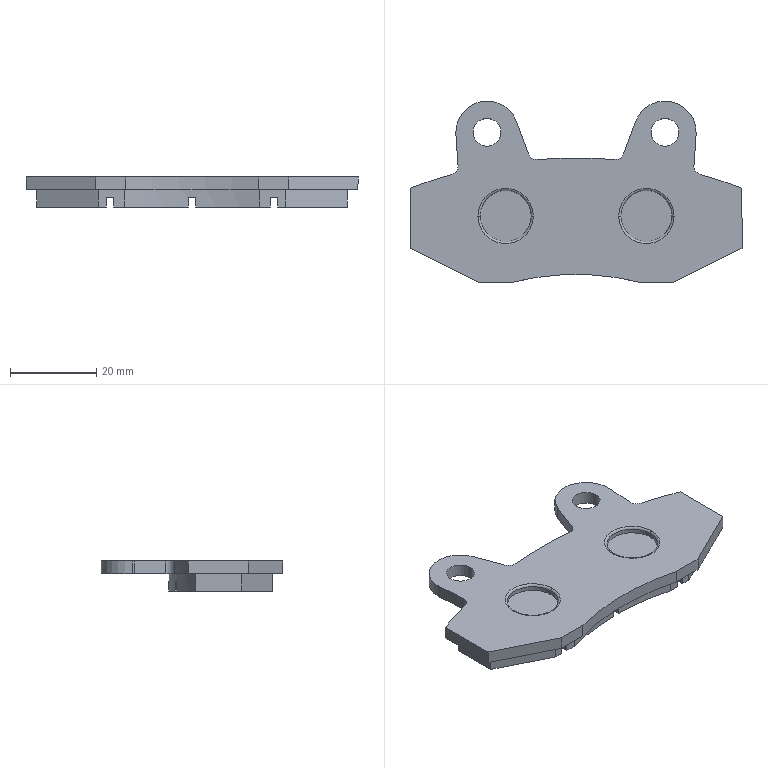Part | SolidWorks | features BaseBody 2 | 2 solids | 60 faces | box 77 x 42.2 x 7 mm | volume 11866 mm3 | plane 34 | cylinder 22 | torus 4 | commonest cylinder face diameters 4 x5 6.45 x4 11.85 x4 14.5 x3 218.75 x3 120.203 x1